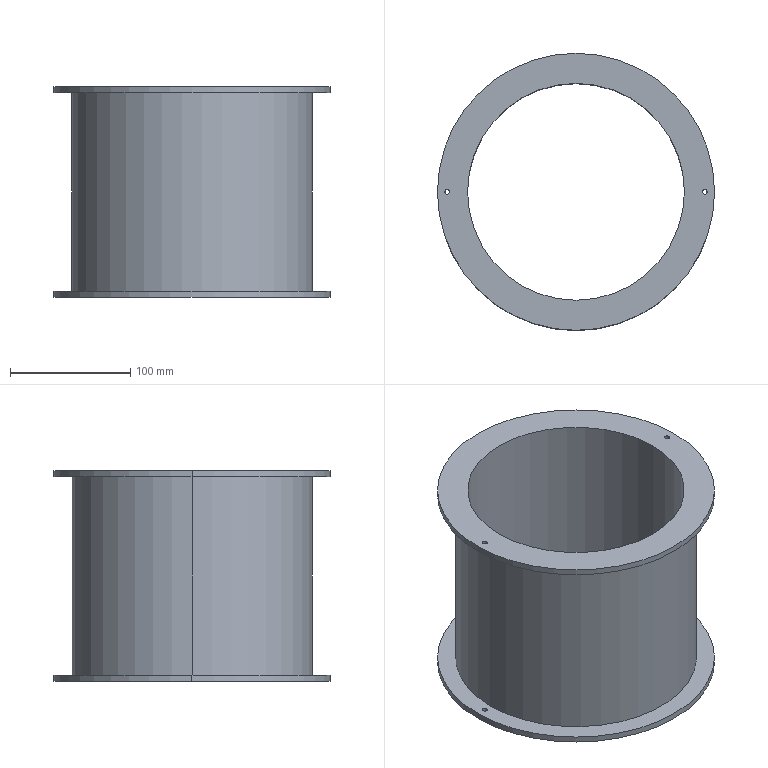Part | STEP file | Housing | 1 solid | 20 faces | box 230 x 230 x 175 mm | volume 1145645 mm3 | cylinder 16 | plane 4 | commonest cylinder face diameters 4 x8 230 x4 180 x2 200 x2
STEP:
#1=CARTESIAN_POINT('',(109.,0.,170.));
#2=VERTEX_POINT('',#1);
#3=CARTESIAN_POINT('',(105.,0.,170.));
#4=VERTEX_POINT('',#3);
#5=CARTESIAN_POINT('',(107.,0.,170.));
#6=DIRECTION('',(0.,0.,-1.));
#7=DIRECTION('',(-1.,0.,0.));
#8=AXIS2_PLACEMENT_3D('',#5,#6,#7);
#9=CIRCLE('',#8,2.);
#10=EDGE_CURVE('',#2,#4,#9,.T.);
#11=ORIENTED_EDGE('',*,*,#10,.F.);
#12=CARTESIAN_POINT('',(109.,0.,165.));
#13=VERTEX_POINT('',#12);
#14=CARTESIAN_POINT('',(109.,0.,170.));
#15=DIRECTION('',(0.,0.,-1.));
#16=VECTOR('',#15,1000.);
#17=LINE('',#14,#16);
#18=EDGE_CURVE('',#2,#13,#17,.T.);
#19=ORIENTED_EDGE('',*,*,#18,.T.);
#20=CARTESIAN_POINT('',(105.,0.,165.));
#21=VERTEX_POINT('',#20);
#22=CARTESIAN_POINT('',(107.,0.,165.));
#23=DIRECTION('',(0.,0.,1.));
#24=DIRECTION('',(1.,0.,0.));
#25=AXIS2_PLACEMENT_3D('',#22,#23,#24);
#26=CIRCLE('',#25,2.);
#27=EDGE_CURVE('',#21,#13,#26,.T.);
#28=ORIENTED_EDGE('',*,*,#27,.F.);
#29=CARTESIAN_POINT('',(105.,0.,170.));
#30=DIRECTION('',(0.,0.,-1.));
#31=VECTOR('',#30,1000.);
#32=LINE('',#29,#31);
#33=EDGE_CURVE('',#4,#21,#32,.T.);
#34=ORIENTED_EDGE('',*,*,#33,.F.);
#35=EDGE_LOOP('',(#11,#19,#28,#34));
#36=FACE_OUTER_BOUND('',#35,.T.);
#37=CARTESIAN_POINT('',(107.,0.,170.));
#38=DIRECTION('',(0.,0.,-1.));
#39=DIRECTION('',(-1.,0.,0.));
#40=AXIS2_PLACEMENT_3D('',#37,#38,#39);
#41=CYLINDRICAL_SURFACE('',#40,2.);
#42=ADVANCED_FACE('',(#36),#41,.F.);
#43=CARTESIAN_POINT('',(-105.,0.,170.));
#44=VERTEX_POINT('',#43);
#45=CARTESIAN_POINT('',(-109.,0.,170.));
#46=VERTEX_POINT('',#45);
#47=CARTESIAN_POINT('',(-107.,0.,170.));
#48=DIRECTION('',(0.,0.,-1.));
#49=DIRECTION('',(-1.,0.,0.));
#50=AXIS2_PLACEMENT_3D('',#47,#48,#49);
#51=CIRCLE('',#50,2.);
#52=EDGE_CURVE('',#44,#46,#51,.T.);
#53=ORIENTED_EDGE('',*,*,#52,.F.);
#54=CARTESIAN_POINT('',(-105.,0.,165.));
#55=VERTEX_POINT('',#54);
#56=CARTESIAN_POINT('',(-105.,0.,170.));
#57=DIRECTION('',(0.,0.,-1.));
#58=VECTOR('',#57,1000.);
#59=LINE('',#56,#58);
#60=EDGE_CURVE('',#44,#55,#59,.T.);
#61=ORIENTED_EDGE('',*,*,#60,.T.);
#62=CARTESIAN_POINT('',(-109.,0.,165.));
#63=VERTEX_POINT('',#62);
#64=CARTESIAN_POINT('',(-107.,0.,165.));
#65=DIRECTION('',(0.,0.,1.));
#66=DIRECTION('',(1.,0.,0.));
#67=AXIS2_PLACEMENT_3D('',#64,#65,#66);
#68=CIRCLE('',#67,2.);
#69=EDGE_CURVE('',#63,#55,#68,.T.);
#70=ORIENTED_EDGE('',*,*,#69,.F.);
#71=CARTESIAN_POINT('',(-109.,0.,170.));
#72=DIRECTION('',(0.,0.,-1.));
#73=VECTOR('',#72,1000.);
#74=LINE('',#71,#73);
#75=EDGE_CURVE('',#46,#63,#74,.T.);
#76=ORIENTED_EDGE('',*,*,#75,.F.);
#77=EDGE_LOOP('',(#53,#61,#70,#76));
#78=FACE_OUTER_BOUND('',#77,.T.);
#79=CARTESIAN_POINT('',(-107.,0.,170.));
#80=DIRECTION('',(0.,0.,-1.));
#81=DIRECTION('',(-1.,0.,0.));
#82=AXIS2_PLACEMENT_3D('',#79,#80,#81);
#83=CYLINDRICAL_SURFACE('',#82,2.);
#84=ADVANCED_FACE('',(#78),#83,.F.);
#85=CARTESIAN_POINT('',(109.,0.,0.));
#86=VERTEX_POINT('',#85);
#87=CARTESIAN_POINT('',(105.,0.,0.));
#88=VERTEX_POINT('',#87);
#89=CARTESIAN_POINT('',(107.,0.,0.));
#90=DIRECTION('',(0.,0.,-1.));
#91=DIRECTION('',(-1.,0.,0.));
#92=AXIS2_PLACEMENT_3D('',#89,#90,#91);
#93=CIRCLE('',#92,2.);
#94=EDGE_CURVE('',#86,#88,#93,.T.);
#95=ORIENTED_EDGE('',*,*,#94,.F.);
#96=CARTESIAN_POINT('',(109.,0.,-5.));
#97=VERTEX_POINT('',#96);
#98=CARTESIAN_POINT('',(109.,0.,170.));
#99=DIRECTION('',(0.,0.,-1.));
#100=VECTOR('',#99,1000.);
#101=LINE('',#98,#100);
#102=EDGE_CURVE('',#86,#97,#101,.T.);
#103=ORIENTED_EDGE('',*,*,#102,.T.);
#104=CARTESIAN_POINT('',(105.,0.,-5.));
#105=VERTEX_POINT('',#104);
#106=CARTESIAN_POINT('',(107.,0.,-5.));
#107=DIRECTION('',(0.,0.,-1.));
#108=DIRECTION('',(-1.,0.,0.));
#109=AXIS2_PLACEMENT_3D('',#106,#107,#108);
#110=CIRCLE('',#109,2.);
#111=EDGE_CURVE('',#97,#105,#110,.T.);
#112=ORIENTED_EDGE('',*,*,#111,.T.);
#113=CARTESIAN_POINT('',(105.,0.,170.));
#114=DIRECTION('',(0.,0.,-1.));
#115=VECTOR('',#114,1000.);
#116=LINE('',#113,#115);
#117=EDGE_CURVE('',#88,#105,#116,.T.);
#118=ORIENTED_EDGE('',*,*,#117,.F.);
#119=EDGE_LOOP('',(#95,#103,#112,#118));
#120=FACE_OUTER_BOUND('',#119,.T.);
#121=CARTESIAN_POINT('',(107.,0.,170.));
#122=DIRECTION('',(0.,0.,-1.));
#123=DIRECTION('',(-1.,0.,0.));
#124=AXIS2_PLACEMENT_3D('',#121,#122,#123);
#125=CYLINDRICAL_SURFACE('',#124,2.);
#126=ADVANCED_FACE('',(#120),#125,.F.);
#127=CARTESIAN_POINT('',(-105.,0.,0.));
#128=VERTEX_POINT('',#127);
#129=CARTESIAN_POINT('',(-109.,0.,0.));
#130=VERTEX_POINT('',#129);
#131=CARTESIAN_POINT('',(-107.,0.,0.));
#132=DIRECTION('',(0.,0.,-1.));
#133=DIRECTION('',(-1.,0.,0.));
#134=AXIS2_PLACEMENT_3D('',#131,#132,#133);
#135=CIRCLE('',#134,2.);
#136=EDGE_CURVE('',#128,#130,#135,.T.);
#137=ORIENTED_EDGE('',*,*,#136,.F.);
#138=CARTESIAN_POINT('',(-105.,0.,-5.));
#139=VERTEX_POINT('',#138);
#140=CARTESIAN_POINT('',(-105.,0.,170.));
#141=DIRECTION('',(0.,0.,-1.));
#142=VECTOR('',#141,1000.);
#143=LINE('',#140,#142);
#144=EDGE_CURVE('',#128,#139,#143,.T.);
#145=ORIENTED_EDGE('',*,*,#144,.T.);
#146=CARTESIAN_POINT('',(-109.,0.,-5.));
#147=VERTEX_POINT('',#146);
#148=CARTESIAN_POINT('',(-107.,0.,-5.));
#149=DIRECTION('',(0.,0.,-1.));
#150=DIRECTION('',(-1.,0.,0.));
#151=AXIS2_PLACEMENT_3D('',#148,#149,#150);
#152=CIRCLE('',#151,2.);
#153=EDGE_CURVE('',#139,#147,#152,.T.);
#154=ORIENTED_EDGE('',*,*,#153,.T.);
#155=CARTESIAN_POINT('',(-109.,0.,170.));
#156=DIRECTION('',(0.,0.,-1.));
#157=VECTOR('',#156,1000.);
#158=LINE('',#155,#157);
#159=EDGE_CURVE('',#130,#147,#158,.T.);
#160=ORIENTED_EDGE('',*,*,#159,.F.);
#161=EDGE_LOOP('',(#137,#145,#154,#160));
#162=FACE_OUTER_BOUND('',#161,.T.);
#163=CARTESIAN_POINT('',(-107.,0.,170.));
#164=DIRECTION('',(0.,0.,-1.));
#165=DIRECTION('',(-1.,0.,0.));
#166=AXIS2_PLACEMENT_3D('',#163,#164,#165);
#167=CYLINDRICAL_SURFACE('',#166,2.);
#168=ADVANCED_FACE('',(#162),#167,.F.);
#169=CARTESIAN_POINT('',(-115.,0.,-5.));
#170=VERTEX_POINT('',#169);
#171=CARTESIAN_POINT('',(115.,0.,-5.));
#172=VERTEX_POINT('',#171);
#173=CARTESIAN_POINT('',(0.,0.,-5.));
#174=DIRECTION('',(0.,0.,-1.));
#175=DIRECTION('',(-1.,0.,0.));
#176=AXIS2_PLACEMENT_3D('',#173,#174,#175);
#177=CIRCLE('',#176,115.);
#178=EDGE_CURVE('',#170,#172,#177,.T.);
#179=ORIENTED_EDGE('',*,*,#178,.F.);
#180=CARTESIAN_POINT('',(-115.,0.,0.));
#181=VERTEX_POINT('',#180);
#182=CARTESIAN_POINT('',(-115.,0.,-5.));
#183=DIRECTION('',(0.,0.,1.));
#184=VECTOR('',#183,1000.);
#185=LINE('',#182,#184);
#186=EDGE_CURVE('',#170,#181,#185,.T.);
#187=ORIENTED_EDGE('',*,*,#186,.T.);
#188=CARTESIAN_POINT('',(115.,0.,0.));
#189=VERTEX_POINT('',#188);
#190=CARTESIAN_POINT('',(0.,0.,0.));
#191=DIRECTION('',(0.,0.,-1.));
#192=DIRECTION('',(-1.,0.,0.));
#193=AXIS2_PLACEMENT_3D('',#190,#191,#192);
#194=CIRCLE('',#193,115.);
#195=EDGE_CURVE('',#181,#189,#194,.T.);
#196=ORIENTED_EDGE('',*,*,#195,.T.);
#197=CARTESIAN_POINT('',(115.,0.,-5.));
#198=DIRECTION('',(0.,0.,1.));
#199=VECTOR('',#198,1000.);
#200=LINE('',#197,#199);
#201=EDGE_CURVE('',#172,#189,#200,.T.);
#202=ORIENTED_EDGE('',*,*,#201,.F.);
#203=EDGE_LOOP('',(#179,#187,#196,#202));
#204=FACE_OUTER_BOUND('',#203,.T.);
#205=CARTESIAN_POINT('',(0.,0.,-5.));
#206=DIRECTION('',(0.,0.,1.));
#207=DIRECTION('',(1.,0.,0.));
#208=AXIS2_PLACEMENT_3D('',#205,#206,#207);
#209=CYLINDRICAL_SURFACE('',#208,115.);
#210=ADVANCED_FACE('',(#204),#209,.T.);
#211=CARTESIAN_POINT('',(115.,0.,170.));
#212=VERTEX_POINT('',#211);
#213=CARTESIAN_POINT('',(-115.,0.,170.));
#214=VERTEX_POINT('',#213);
#215=CARTESIAN_POINT('',(0.,0.,170.));
#216=DIRECTION('',(0.,0.,1.));
#217=DIRECTION('',(1.,0.,0.));
#218=AXIS2_PLACEMENT_3D('',#215,#216,#217);
#219=CIRCLE('',#218,115.);
#220=EDGE_CURVE('',#212,#214,#219,.T.);
#221=ORIENTED_EDGE('',*,*,#220,.F.);
#222=CARTESIAN_POINT('',(115.,0.,165.));
#223=VERTEX_POINT('',#222);
#224=CARTESIAN_POINT('',(115.,0.,170.));
#225=DIRECTION('',(0.,0.,-1.));
#226=VECTOR('',#225,1000.);
#227=LINE('',#224,#226);
#228=EDGE_CURVE('',#212,#223,#227,.T.);
#229=ORIENTED_EDGE('',*,*,#228,.T.);
#230=CARTESIAN_POINT('',(-115.,0.,165.));
#231=VERTEX_POINT('',#230);
#232=CARTESIAN_POINT('',(0.,0.,165.));
#233=DIRECTION('',(0.,0.,1.));
#234=DIRECTION('',(1.,0.,0.));
#235=AXIS2_PLACEMENT_3D('',#232,#233,#234);
#236=CIRCLE('',#235,115.);
#237=EDGE_CURVE('',#223,#231,#236,.T.);
#238=ORIENTED_EDGE('',*,*,#237,.T.);
#239=CARTESIAN_POINT('',(-115.,0.,170.));
#240=DIRECTION('',(0.,0.,-1.));
#241=VECTOR('',#240,1000.);
#242=LINE('',#239,#241);
#243=EDGE_CURVE('',#214,#231,#242,.T.);
#244=ORIENTED_EDGE('',*,*,#243,.F.);
#245=EDGE_LOOP('',(#221,#229,#238,#244));
#246=FACE_OUTER_BOUND('',#245,.T.);
#247=CARTESIAN_POINT('',(0.,0.,170.));
#248=DIRECTION('',(0.,0.,-1.));
#249=DIRECTION('',(-1.,0.,0.));
#250=AXIS2_PLACEMENT_3D('',#247,#248,#249);
#251=CYLINDRICAL_SURFACE('',#250,115.);
#252=ADVANCED_FACE('',(#246),#251,.T.);
#253=CARTESIAN_POINT('',(-90.,0.,170.));
#254=VERTEX_POINT('',#253);
#255=CARTESIAN_POINT('',(90.,0.,170.));
#256=VERTEX_POINT('',#255);
#257=CARTESIAN_POINT('',(0.,0.,170.));
#258=DIRECTION('',(0.,0.,1.));
#259=DIRECTION('',(1.,0.,0.));
#260=AXIS2_PLACEMENT_3D('',#257,#258,#259);
#261=CIRCLE('',#260,90.);
#262=EDGE_CURVE('',#254,#256,#261,.T.);
#263=ORIENTED_EDGE('',*,*,#262,.T.);
#264=CARTESIAN_POINT('',(90.,0.,-5.));
#265=VERTEX_POINT('',#264);
#266=CARTESIAN_POINT('',(90.,0.,165.));
#267=DIRECTION('',(0.,0.,-1.));
#268=VECTOR('',#267,1000.);
#269=LINE('',#266,#268);
#270=EDGE_CURVE('',#256,#265,#269,.T.);
#271=ORIENTED_EDGE('',*,*,#270,.T.);
#272=CARTESIAN_POINT('',(-90.,0.,-5.));
#273=VERTEX_POINT('',#272);
#274=CARTESIAN_POINT('',(0.,0.,-5.));
#275=DIRECTION('',(0.,0.,-1.));
#276=DIRECTION('',(-1.,0.,0.));
#277=AXIS2_PLACEMENT_3D('',#274,#275,#276);
#278=CIRCLE('',#277,90.);
#279=EDGE_CURVE('',#265,#273,#278,.T.);
#280=ORIENTED_EDGE('',*,*,#279,.T.);
#281=CARTESIAN_POINT('',(-90.,0.,165.));
#282=DIRECTION('',(0.,0.,-1.));
#283=VECTOR('',#282,1000.);
#284=LINE('',#281,#283);
#285=EDGE_CURVE('',#254,#273,#284,.T.);
#286=ORIENTED_EDGE('',*,*,#285,.F.);
#287=EDGE_LOOP('',(#263,#271,#280,#286));
#288=FACE_OUTER_BOUND('',#287,.T.);
#289=CARTESIAN_POINT('',(0.,0.,165.));
#290=DIRECTION('',(0.,0.,-1.));
#291=DIRECTION('',(-1.,0.,0.));
#292=AXIS2_PLACEMENT_3D('',#289,#290,#291);
#293=CYLINDRICAL_SURFACE('',#292,90.);
#294=ADVANCED_FACE('',(#288),#293,.F.);
#295=CARTESIAN_POINT('',(100.,0.,165.));
#296=VERTEX_POINT('',#295);
#297=CARTESIAN_POINT('',(-100.,0.,165.));
#298=VERTEX_POINT('',#297);
#299=CARTESIAN_POINT('',(0.,0.,165.));
#300=DIRECTION('',(0.,0.,1.));
#301=DIRECTION('',(1.,0.,0.));
#302=AXIS2_PLACEMENT_3D('',#299,#300,#301);
#303=CIRCLE('',#302,100.);
#304=EDGE_CURVE('',#296,#298,#303,.T.);
#305=ORIENTED_EDGE('',*,*,#304,.F.);
#306=CARTESIAN_POINT('',(100.,0.,0.));
#307=VERTEX_POINT('',#306);
#308=CARTESIAN_POINT('',(100.,0.,165.));
#309=DIRECTION('',(0.,0.,-1.));
#310=VECTOR('',#309,1000.);
#311=LINE('',#308,#310);
#312=EDGE_CURVE('',#296,#307,#311,.T.);
#313=ORIENTED_EDGE('',*,*,#312,.T.);
#314=CARTESIAN_POINT('',(-100.,0.,0.));
#315=VERTEX_POINT('',#314);
#316=CARTESIAN_POINT('',(0.,0.,0.));
#317=DIRECTION('',(0.,0.,1.));
#318=DIRECTION('',(1.,0.,0.));
#319=AXIS2_PLACEMENT_3D('',#316,#317,#318);
#320=CIRCLE('',#319,100.);
#321=EDGE_CURVE('',#307,#315,#320,.T.);
#322=ORIENTED_EDGE('',*,*,#321,.T.);
#323=CARTESIAN_POINT('',(-100.,0.,165.));
#324=DIRECTION('',(0.,0.,-1.));
#325=VECTOR('',#324,1000.);
#326=LINE('',#323,#325);
#327=EDGE_CURVE('',#298,#315,#326,.T.);
#328=ORIENTED_EDGE('',*,*,#327,.F.);
#329=EDGE_LOOP('',(#305,#313,#322,#328));
#330=FACE_OUTER_BOUND('',#329,.T.);
#331=CARTESIAN_POINT('',(0.,0.,165.));
#332=DIRECTION('',(0.,0.,-1.));
#333=DIRECTION('',(-1.,0.,0.));
#334=AXIS2_PLACEMENT_3D('',#331,#332,#333);
#335=CYLINDRICAL_SURFACE('',#334,100.);
#336=ADVANCED_FACE('',(#330),#335,.T.);
#337=ORIENTED_EDGE('',*,*,#312,.F.);
#338=CARTESIAN_POINT('',(0.,0.,165.));
#339=DIRECTION('',(0.,0.,1.));
#340=DIRECTION('',(1.,0.,0.));
#341=AXIS2_PLACEMENT_3D('',#338,#339,#340);
#342=CIRCLE('',#341,100.);
#343=EDGE_CURVE('',#298,#296,#342,.T.);
#344=ORIENTED_EDGE('',*,*,#343,.F.);
#345=ORIENTED_EDGE('',*,*,#327,.T.);
#346=CARTESIAN_POINT('',(0.,0.,0.));
#347=DIRECTION('',(0.,0.,1.));
#348=DIRECTION('',(1.,0.,0.));
#349=AXIS2_PLACEMENT_3D('',#346,#347,#348);
#350=CIRCLE('',#349,100.);
#351=EDGE_CURVE('',#315,#307,#350,.T.);
#352=ORIENTED_EDGE('',*,*,#351,.T.);
#353=EDGE_LOOP('',(#337,#344,#345,#352));
#354=FACE_OUTER_BOUND('',#353,.T.);
#355=CARTESIAN_POINT('',(0.,0.,165.));
#356=DIRECTION('',(0.,0.,-1.));
#357=DIRECTION('',(-1.,0.,0.));
#358=AXIS2_PLACEMENT_3D('',#355,#356,#357);
#359=CYLINDRICAL_SURFACE('',#358,100.);
#360=ADVANCED_FACE('',(#354),#359,.T.);
#361=ORIENTED_EDGE('',*,*,#270,.F.);
#362=CARTESIAN_POINT('',(0.,0.,170.));
#363=DIRECTION('',(0.,0.,1.));
#364=DIRECTION('',(1.,0.,0.));
#365=AXIS2_PLACEMENT_3D('',#362,#363,#364);
#366=CIRCLE('',#365,90.);
#367=EDGE_CURVE('',#256,#254,#366,.T.);
#368=ORIENTED_EDGE('',*,*,#367,.T.);
#369=ORIENTED_EDGE('',*,*,#285,.T.);
#370=CARTESIAN_POINT('',(0.,0.,-5.));
#371=DIRECTION('',(0.,0.,-1.));
#372=DIRECTION('',(-1.,0.,0.));
#373=AXIS2_PLACEMENT_3D('',#370,#371,#372);
#374=CIRCLE('',#373,90.);
#375=EDGE_CURVE('',#273,#265,#374,.T.);
#376=ORIENTED_EDGE('',*,*,#375,.T.);
#377=EDGE_LOOP('',(#361,#368,#369,#376));
#378=FACE_OUTER_BOUND('',#377,.T.);
#379=CARTESIAN_POINT('',(0.,0.,165.));
#380=DIRECTION('',(0.,0.,-1.));
#381=DIRECTION('',(-1.,0.,0.));
#382=AXIS2_PLACEMENT_3D('',#379,#380,#381);
#383=CYLINDRICAL_SURFACE('',#382,90.);
#384=ADVANCED_FACE('',(#378),#383,.F.);
#385=CARTESIAN_POINT('',(107.,0.,170.));
#386=DIRECTION('',(0.,0.,-1.));
#387=DIRECTION('',(-1.,0.,0.));
#388=AXIS2_PLACEMENT_3D('',#385,#386,#387);
#389=CIRCLE('',#388,2.);
#390=EDGE_CURVE('',#4,#2,#389,.T.);
#391=ORIENTED_EDGE('',*,*,#390,.T.);
#392=ORIENTED_EDGE('',*,*,#10,.T.);
#393=EDGE_LOOP('',(#391,#392));
#394=FACE_BOUND('',#393,.T.);
#395=CARTESIAN_POINT('',(-107.,0.,170.));
#396=DIRECTION('',(0.,0.,-1.));
#397=DIRECTION('',(-1.,0.,0.));
#398=AXIS2_PLACEMENT_3D('',#395,#396,#397);
#399=CIRCLE('',#398,2.);
#400=EDGE_CURVE('',#46,#44,#399,.T.);
#401=ORIENTED_EDGE('',*,*,#400,.T.);
#402=ORIENTED_EDGE('',*,*,#52,.T.);
#403=EDGE_LOOP('',(#401,#402));
#404=FACE_BOUND('',#403,.T.);
#405=CARTESIAN_POINT('',(0.,0.,170.));
#406=DIRECTION('',(0.,0.,1.));
#407=DIRECTION('',(1.,0.,0.));
#408=AXIS2_PLACEMENT_3D('',#405,#406,#407);
#409=CIRCLE('',#408,115.);
#410=EDGE_CURVE('',#214,#212,#409,.T.);
#411=ORIENTED_EDGE('',*,*,#410,.T.);
#412=ORIENTED_EDGE('',*,*,#220,.T.);
#413=EDGE_LOOP('',(#411,#412));
#414=FACE_OUTER_BOUND('',#413,.T.);
#415=ORIENTED_EDGE('',*,*,#262,.F.);
#416=ORIENTED_EDGE('',*,*,#367,.F.);
#417=EDGE_LOOP('',(#415,#416));
#418=FACE_BOUND('',#417,.T.);
#419=CARTESIAN_POINT('',(0.,0.,170.));
#420=DIRECTION('',(0.,0.,1.));
#421=DIRECTION('',(1.,0.,0.));
#422=AXIS2_PLACEMENT_3D('',#419,#420,#421);
#423=PLANE('',#422);
#424=ADVANCED_FACE('',(#394,#404,#414,#418),#423,.T.);
#425=ORIENTED_EDGE('',*,*,#27,.T.);
#426=CARTESIAN_POINT('',(107.,0.,165.));
#427=DIRECTION('',(0.,0.,1.));
#428=DIRECTION('',(1.,0.,0.));
#429=AXIS2_PLACEMENT_3D('',#426,#427,#428);
#430=CIRCLE('',#429,2.);
#431=EDGE_CURVE('',#13,#21,#430,.T.);
#432=ORIENTED_EDGE('',*,*,#431,.T.);
#433=EDGE_LOOP('',(#425,#432));
#434=FACE_BOUND('',#433,.T.);
#435=ORIENTED_EDGE('',*,*,#69,.T.);
#436=CARTESIAN_POINT('',(-107.,0.,165.));
#437=DIRECTION('',(0.,0.,1.));
#438=DIRECTION('',(1.,0.,0.));
#439=AXIS2_PLACEMENT_3D('',#436,#437,#438);
#440=CIRCLE('',#439,2.);
#441=EDGE_CURVE('',#55,#63,#440,.T.);
#442=ORIENTED_EDGE('',*,*,#441,.T.);
#443=EDGE_LOOP('',(#435,#442));
#444=FACE_BOUND('',#443,.T.);
#445=ORIENTED_EDGE('',*,*,#343,.T.);
#446=ORIENTED_EDGE('',*,*,#304,.T.);
#447=EDGE_LOOP('',(#445,#446));
#448=FACE_BOUND('',#447,.T.);
#449=CARTESIAN_POINT('',(0.,0.,165.));
#450=DIRECTION('',(0.,0.,1.));
#451=DIRECTION('',(1.,0.,0.));
#452=AXIS2_PLACEMENT_3D('',#449,#450,#451);
#453=CIRCLE('',#452,115.);
#454=EDGE_CURVE('',#231,#223,#453,.T.);
#455=ORIENTED_EDGE('',*,*,#454,.F.);
#456=ORIENTED_EDGE('',*,*,#237,.F.);
#457=EDGE_LOOP('',(#455,#456));
#458=FACE_OUTER_BOUND('',#457,.T.);
#459=CARTESIAN_POINT('',(0.,0.,165.));
#460=DIRECTION('',(0.,0.,1.));
#461=DIRECTION('',(1.,0.,0.));
#462=AXIS2_PLACEMENT_3D('',#459,#460,#461);
#463=PLANE('',#462);
#464=ADVANCED_FACE('',(#434,#444,#448,#458),#463,.F.);
#465=ORIENTED_EDGE('',*,*,#228,.F.);
#466=ORIENTED_EDGE('',*,*,#410,.F.);
#467=ORIENTED_EDGE('',*,*,#243,.T.);
#468=ORIENTED_EDGE('',*,*,#454,.T.);
#469=EDGE_LOOP('',(#465,#466,#467,#468));
#470=FACE_OUTER_BOUND('',#469,.T.);
#471=CARTESIAN_POINT('',(0.,0.,170.));
#472=DIRECTION('',(0.,0.,-1.));
#473=DIRECTION('',(-1.,0.,0.));
#474=AXIS2_PLACEMENT_3D('',#471,#472,#473);
#475=CYLINDRICAL_SURFACE('',#474,115.);
#476=ADVANCED_FACE('',(#470),#475,.T.);
#477=CARTESIAN_POINT('',(107.,0.,-5.));
#478=DIRECTION('',(0.,0.,-1.));
#479=DIRECTION('',(-1.,0.,0.));
#480=AXIS2_PLACEMENT_3D('',#477,#478,#479);
#481=CIRCLE('',#480,2.);
#482=EDGE_CURVE('',#105,#97,#481,.T.);
#483=ORIENTED_EDGE('',*,*,#482,.F.);
#484=ORIENTED_EDGE('',*,*,#111,.F.);
#485=EDGE_LOOP('',(#483,#484));
#486=FACE_BOUND('',#485,.T.);
#487=CARTESIAN_POINT('',(-107.,0.,-5.));
#488=DIRECTION('',(0.,0.,-1.));
#489=DIRECTION('',(-1.,0.,0.));
#490=AXIS2_PLACEMENT_3D('',#487,#488,#489);
#491=CIRCLE('',#490,2.);
#492=EDGE_CURVE('',#147,#139,#491,.T.);
#493=ORIENTED_EDGE('',*,*,#492,.F.);
#494=ORIENTED_EDGE('',*,*,#153,.F.);
#495=EDGE_LOOP('',(#493,#494));
#496=FACE_BOUND('',#495,.T.);
#497=CARTESIAN_POINT('',(0.,0.,-5.));
#498=DIRECTION('',(0.,0.,-1.));
#499=DIRECTION('',(-1.,0.,0.));
#500=AXIS2_PLACEMENT_3D('',#497,#498,#499);
#501=CIRCLE('',#500,115.);
#502=EDGE_CURVE('',#172,#170,#501,.T.);
#503=ORIENTED_EDGE('',*,*,#502,.T.);
#504=ORIENTED_EDGE('',*,*,#178,.T.);
#505=EDGE_LOOP('',(#503,#504));
#506=FACE_OUTER_BOUND('',#505,.T.);
#507=ORIENTED_EDGE('',*,*,#375,.F.);
#508=ORIENTED_EDGE('',*,*,#279,.F.);
#509=EDGE_LOOP('',(#507,#508));
#510=FACE_BOUND('',#509,.T.);
#511=CARTESIAN_POINT('',(0.,0.,-5.));
#512=DIRECTION('',(0.,0.,-1.));
#513=DIRECTION('',(-1.,0.,0.));
#514=AXIS2_PLACEMENT_3D('',#511,#512,#513);
#515=PLANE('',#514);
#516=ADVANCED_FACE('',(#486,#496,#506,#510),#515,.T.);
#517=CARTESIAN_POINT('',(107.,0.,0.));
#518=DIRECTION('',(0.,0.,-1.));
#519=DIRECTION('',(-1.,0.,0.));
#520=AXIS2_PLACEMENT_3D('',#517,#518,#519);
#521=CIRCLE('',#520,2.);
#522=EDGE_CURVE('',#88,#86,#521,.T.);
#523=ORIENTED_EDGE('',*,*,#522,.T.);
#524=ORIENTED_EDGE('',*,*,#94,.T.);
#525=EDGE_LOOP('',(#523,#524));
#526=FACE_BOUND('',#525,.T.);
#527=CARTESIAN_POINT('',(-107.,0.,0.));
#528=DIRECTION('',(0.,0.,-1.));
#529=DIRECTION('',(-1.,0.,0.));
#530=AXIS2_PLACEMENT_3D('',#527,#528,#529);
#531=CIRCLE('',#530,2.);
#532=EDGE_CURVE('',#130,#128,#531,.T.);
#533=ORIENTED_EDGE('',*,*,#532,.T.);
#534=ORIENTED_EDGE('',*,*,#136,.T.);
#535=EDGE_LOOP('',(#533,#534));
#536=FACE_BOUND('',#535,.T.);
#537=ORIENTED_EDGE('',*,*,#351,.F.);
#538=ORIENTED_EDGE('',*,*,#321,.F.);
#539=EDGE_LOOP('',(#537,#538));
#540=FACE_BOUND('',#539,.T.);
#541=CARTESIAN_POINT('',(0.,0.,0.));
#542=DIRECTION('',(0.,0.,-1.));
#543=DIRECTION('',(-1.,0.,0.));
#544=AXIS2_PLACEMENT_3D('',#541,#542,#543);
#545=CIRCLE('',#544,115.);
#546=EDGE_CURVE('',#189,#181,#545,.T.);
#547=ORIENTED_EDGE('',*,*,#546,.F.);
#548=ORIENTED_EDGE('',*,*,#195,.F.);
#549=EDGE_LOOP('',(#547,#548));
#550=FACE_OUTER_BOUND('',#549,.T.);
#551=CARTESIAN_POINT('',(0.,0.,0.));
#552=DIRECTION('',(0.,0.,-1.));
#553=DIRECTION('',(-1.,0.,0.));
#554=AXIS2_PLACEMENT_3D('',#551,#552,#553);
#555=PLANE('',#554);
#556=ADVANCED_FACE('',(#526,#536,#540,#550),#555,.F.);
#557=ORIENTED_EDGE('',*,*,#186,.F.);
#558=ORIENTED_EDGE('',*,*,#502,.F.);
#559=ORIENTED_EDGE('',*,*,#201,.T.);
#560=ORIENTED_EDGE('',*,*,#546,.T.);
#561=EDGE_LOOP('',(#557,#558,#559,#560));
#562=FACE_OUTER_BOUND('',#561,.T.);
#563=CARTESIAN_POINT('',(0.,0.,-5.));
#564=DIRECTION('',(0.,0.,1.));
#565=DIRECTION('',(1.,0.,0.));
#566=AXIS2_PLACEMENT_3D('',#563,#564,#565);
#567=CYLINDRICAL_SURFACE('',#566,115.);
#568=ADVANCED_FACE('',(#562),#567,.T.);
#569=ORIENTED_EDGE('',*,*,#144,.F.);
#570=ORIENTED_EDGE('',*,*,#532,.F.);
#571=ORIENTED_EDGE('',*,*,#159,.T.);
#572=ORIENTED_EDGE('',*,*,#492,.T.);
#573=EDGE_LOOP('',(#569,#570,#571,#572));
#574=FACE_OUTER_BOUND('',#573,.T.);
#575=CARTESIAN_POINT('',(-107.,0.,170.));
#576=DIRECTION('',(0.,0.,-1.));
#577=DIRECTION('',(-1.,0.,0.));
#578=AXIS2_PLACEMENT_3D('',#575,#576,#577);
#579=CYLINDRICAL_SURFACE('',#578,2.);
#580=ADVANCED_FACE('',(#574),#579,.F.);
#581=ORIENTED_EDGE('',*,*,#102,.F.);
#582=ORIENTED_EDGE('',*,*,#522,.F.);
#583=ORIENTED_EDGE('',*,*,#117,.T.);
#584=ORIENTED_EDGE('',*,*,#482,.T.);
#585=EDGE_LOOP('',(#581,#582,#583,#584));
#586=FACE_OUTER_BOUND('',#585,.T.);
#587=CARTESIAN_POINT('',(107.,0.,170.));
#588=DIRECTION('',(0.,0.,-1.));
#589=DIRECTION('',(-1.,0.,0.));
#590=AXIS2_PLACEMENT_3D('',#587,#588,#589);
#591=CYLINDRICAL_SURFACE('',#590,2.);
#592=ADVANCED_FACE('',(#586),#591,.F.);
#593=ORIENTED_EDGE('',*,*,#60,.F.);
#594=ORIENTED_EDGE('',*,*,#400,.F.);
#595=ORIENTED_EDGE('',*,*,#75,.T.);
#596=ORIENTED_EDGE('',*,*,#441,.F.);
#597=EDGE_LOOP('',(#593,#594,#595,#596));
#598=FACE_OUTER_BOUND('',#597,.T.);
#599=CARTESIAN_POINT('',(-107.,0.,170.));
#600=DIRECTION('',(0.,0.,-1.));
#601=DIRECTION('',(-1.,0.,0.));
#602=AXIS2_PLACEMENT_3D('',#599,#600,#601);
#603=CYLINDRICAL_SURFACE('',#602,2.);
#604=ADVANCED_FACE('',(#598),#603,.F.);
#605=ORIENTED_EDGE('',*,*,#18,.F.);
#606=ORIENTED_EDGE('',*,*,#390,.F.);
#607=ORIENTED_EDGE('',*,*,#33,.T.);
#608=ORIENTED_EDGE('',*,*,#431,.F.);
#609=EDGE_LOOP('',(#605,#606,#607,#608));
#610=FACE_OUTER_BOUND('',#609,.T.);
#611=CARTESIAN_POINT('',(107.,0.,170.));
#612=DIRECTION('',(0.,0.,-1.));
#613=DIRECTION('',(-1.,0.,0.));
#614=AXIS2_PLACEMENT_3D('',#611,#612,#613);
#615=CYLINDRICAL_SURFACE('',#614,2.);
#616=ADVANCED_FACE('',(#610),#615,.F.);
#617=CLOSED_SHELL('',(#42,#84,#126,#168,#210,#252,#294,#336,#360,#384,#424,#464,#476,#516,#556,#568,#580,#592,#604,#616));
#618=MANIFOLD_SOLID_BREP('',#617);
#619=CARTESIAN_POINT('',(0.,0.,0.));
#620=DIRECTION('',(0.,0.,1.));
#621=DIRECTION('',(1.,0.,0.));
#622=AXIS2_PLACEMENT_3D('',#619,#620,#621);
#623=(LENGTH_UNIT()NAMED_UNIT(*)SI_UNIT(.MILLI.,.METRE.));
#624=UNCERTAINTY_MEASURE_WITH_UNIT(LENGTH_MEASURE(0.00001),#623,'','');
#625=(NAMED_UNIT(*)PLANE_ANGLE_UNIT()SI_UNIT($,.RADIAN.));
#626=(NAMED_UNIT(*)SI_UNIT($,.STERADIAN.)SOLID_ANGLE_UNIT());
#627=(GEOMETRIC_REPRESENTATION_CONTEXT(3)GLOBAL_UNCERTAINTY_ASSIGNED_CONTEXT((#624))GLOBAL_UNIT_ASSIGNED_CONTEXT((#623,#625,#626))REPRESENTATION_CONTEXT('',''));
#628=ADVANCED_BREP_SHAPE_REPRESENTATION('',(#618,#622),#627);